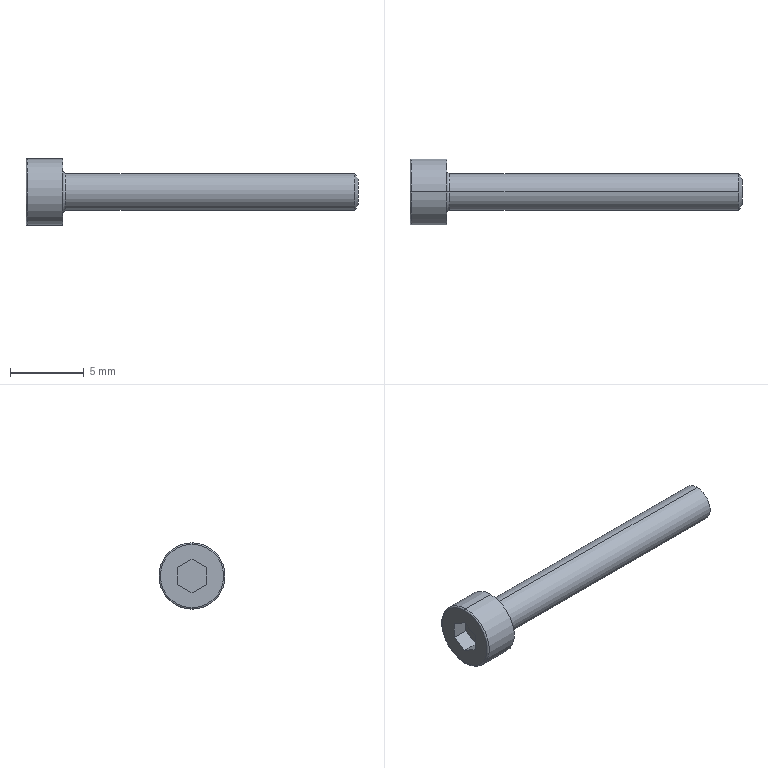Part | SolidWorks | features BlendCut 1, Cut 1, Fillet 1, LPattern 1, RevCut 1, Revolution 1 | 1 solid | 20 faces | box 22.5 x 4.5 x 4.5 mm | volume 133.887 mm3 | plane 10 | torus 4 | cylinder 4 | cone 2 | commonest cylinder face diameters 2.5 x2 4.5 x2
STEP:
#1=CARTESIAN_POINT('',(0.,0.,2.15));
#2=VERTEX_POINT('',#1);
#3=CARTESIAN_POINT('',(0.,0.,-2.15));
#4=VERTEX_POINT('',#3);
#5=CARTESIAN_POINT('',(0.,0.,0.));
#6=DIRECTION('',(-1.,0.,0.));
#7=DIRECTION('',(0.,0.,-1.));
#8=AXIS2_PLACEMENT_3D('',#5,#6,#7);
#9=CIRCLE('',#8,2.15);
#10=EDGE_CURVE('',#2,#4,#9,.T.);
#11=ORIENTED_EDGE('',*,*,#10,.F.);
#12=CARTESIAN_POINT('',(0.1,0.,2.25));
#13=VERTEX_POINT('',#12);
#14=CARTESIAN_POINT('',(0.1,0.,2.15));
#15=DIRECTION('',(0.,1.,0.));
#16=DIRECTION('',(0.,0.,1.));
#17=AXIS2_PLACEMENT_3D('',#14,#15,#16);
#18=CIRCLE('',#17,0.1);
#19=EDGE_CURVE('',#2,#13,#18,.T.);
#20=ORIENTED_EDGE('',*,*,#19,.T.);
#21=CARTESIAN_POINT('',(0.1,0.,-2.25));
#22=VERTEX_POINT('',#21);
#23=CARTESIAN_POINT('',(0.1,0.,0.));
#24=DIRECTION('',(1.,0.,0.));
#25=DIRECTION('',(0.,0.,-1.));
#26=AXIS2_PLACEMENT_3D('',#23,#24,#25);
#27=CIRCLE('',#26,2.25);
#28=EDGE_CURVE('',#22,#13,#27,.T.);
#29=ORIENTED_EDGE('',*,*,#28,.F.);
#30=CARTESIAN_POINT('',(0.1,0.,-2.15));
#31=DIRECTION('',(0.,-1.,0.));
#32=DIRECTION('',(0.,0.,-1.));
#33=AXIS2_PLACEMENT_3D('',#30,#31,#32);
#34=CIRCLE('',#33,0.1);
#35=EDGE_CURVE('',#4,#22,#34,.T.);
#36=ORIENTED_EDGE('',*,*,#35,.F.);
#37=EDGE_LOOP('',(#11,#20,#29,#36));
#38=FACE_OUTER_BOUND('',#37,.T.);
#39=CARTESIAN_POINT('',(0.1,0.,0.));
#40=DIRECTION('',(1.,0.,0.));
#41=DIRECTION('',(0.,0.,-1.));
#42=AXIS2_PLACEMENT_3D('',#39,#40,#41);
#43=TOROIDAL_SURFACE('',#42,2.15,0.1);
#44=ADVANCED_FACE('',(#38),#43,.T.);
#45=CARTESIAN_POINT('',(22.5,0.,0.8603));
#46=VERTEX_POINT('',#45);
#47=CARTESIAN_POINT('',(22.5,0.,-0.8603));
#48=VERTEX_POINT('',#47);
#49=CARTESIAN_POINT('',(22.5,0.,0.));
#50=DIRECTION('',(-1.,0.,0.));
#51=DIRECTION('',(0.,0.,1.));
#52=AXIS2_PLACEMENT_3D('',#49,#50,#51);
#53=CIRCLE('',#52,0.8603);
#54=EDGE_CURVE('',#46,#48,#53,.T.);
#55=ORIENTED_EDGE('',*,*,#54,.T.);
#56=CARTESIAN_POINT('',(22.275,0.,-1.25));
#57=VERTEX_POINT('',#56);
#58=CARTESIAN_POINT('',(22.275,0.,-1.25));
#59=DIRECTION('',(-0.5,0.,-0.866));
#60=VECTOR('',#59,1000.);
#61=LINE('',#58,#60);
#62=EDGE_CURVE('',#48,#57,#61,.T.);
#63=ORIENTED_EDGE('',*,*,#62,.T.);
#64=CARTESIAN_POINT('',(22.275,0.,1.25));
#65=VERTEX_POINT('',#64);
#66=CARTESIAN_POINT('',(22.275,0.,0.));
#67=DIRECTION('',(-1.,0.,0.));
#68=DIRECTION('',(0.,0.,1.));
#69=AXIS2_PLACEMENT_3D('',#66,#67,#68);
#70=CIRCLE('',#69,1.25);
#71=EDGE_CURVE('',#65,#57,#70,.T.);
#72=ORIENTED_EDGE('',*,*,#71,.F.);
#73=CARTESIAN_POINT('',(22.275,0.,1.25));
#74=DIRECTION('',(-0.5,0.,0.866));
#75=VECTOR('',#74,1000.);
#76=LINE('',#73,#75);
#77=EDGE_CURVE('',#46,#65,#76,.T.);
#78=ORIENTED_EDGE('',*,*,#77,.F.);
#79=EDGE_LOOP('',(#55,#63,#72,#78));
#80=FACE_OUTER_BOUND('',#79,.T.);
#81=CARTESIAN_POINT('',(22.275,0.,0.));
#82=DIRECTION('',(-1.,0.,0.));
#83=DIRECTION('',(0.,0.,1.));
#84=AXIS2_PLACEMENT_3D('',#81,#82,#83);
#85=CONICAL_SURFACE('',#84,1.25,1.047);
#86=ADVANCED_FACE('',(#80),#85,.T.);
#87=CARTESIAN_POINT('',(2.5,0.,-1.45));
#88=VERTEX_POINT('',#87);
#89=CARTESIAN_POINT('',(2.5,0.,1.45));
#90=VERTEX_POINT('',#89);
#91=CARTESIAN_POINT('',(2.5,0.,0.));
#92=DIRECTION('',(-1.,0.,0.));
#93=DIRECTION('',(0.,0.,1.));
#94=AXIS2_PLACEMENT_3D('',#91,#92,#93);
#95=CIRCLE('',#94,1.45);
#96=EDGE_CURVE('',#88,#90,#95,.T.);
#97=ORIENTED_EDGE('',*,*,#96,.F.);
#98=CARTESIAN_POINT('',(2.7,0.,-1.25));
#99=VERTEX_POINT('',#98);
#100=CARTESIAN_POINT('',(2.7,0.,-1.45));
#101=DIRECTION('',(0.,1.,0.));
#102=DIRECTION('',(0.,0.,1.));
#103=AXIS2_PLACEMENT_3D('',#100,#101,#102);
#104=CIRCLE('',#103,0.2);
#105=EDGE_CURVE('',#88,#99,#104,.T.);
#106=ORIENTED_EDGE('',*,*,#105,.T.);
#107=CARTESIAN_POINT('',(2.7,0.,1.25));
#108=VERTEX_POINT('',#107);
#109=CARTESIAN_POINT('',(2.7,0.,0.));
#110=DIRECTION('',(-1.,0.,0.));
#111=DIRECTION('',(0.,0.,1.));
#112=AXIS2_PLACEMENT_3D('',#109,#110,#111);
#113=CIRCLE('',#112,1.25);
#114=EDGE_CURVE('',#99,#108,#113,.T.);
#115=ORIENTED_EDGE('',*,*,#114,.T.);
#116=CARTESIAN_POINT('',(2.7,0.,1.45));
#117=DIRECTION('',(0.,-1.,0.));
#118=DIRECTION('',(0.,0.,-1.));
#119=AXIS2_PLACEMENT_3D('',#116,#117,#118);
#120=CIRCLE('',#119,0.2);
#121=EDGE_CURVE('',#90,#108,#120,.T.);
#122=ORIENTED_EDGE('',*,*,#121,.F.);
#123=EDGE_LOOP('',(#97,#106,#115,#122));
#124=FACE_OUTER_BOUND('',#123,.T.);
#125=CARTESIAN_POINT('',(2.7,0.,0.));
#126=DIRECTION('',(-1.,0.,0.));
#127=DIRECTION('',(0.,0.,1.));
#128=AXIS2_PLACEMENT_3D('',#125,#126,#127);
#129=TOROIDAL_SURFACE('',#128,1.45,0.2);
#130=ADVANCED_FACE('',(#124),#129,.F.);
#131=CARTESIAN_POINT('',(2.5,0.,2.25));
#132=VERTEX_POINT('',#131);
#133=CARTESIAN_POINT('',(2.5,0.,-2.25));
#134=VERTEX_POINT('',#133);
#135=CARTESIAN_POINT('',(2.5,0.,0.));
#136=DIRECTION('',(-1.,0.,0.));
#137=DIRECTION('',(0.,0.,1.));
#138=AXIS2_PLACEMENT_3D('',#135,#136,#137);
#139=CIRCLE('',#138,2.25);
#140=EDGE_CURVE('',#132,#134,#139,.T.);
#141=ORIENTED_EDGE('',*,*,#140,.T.);
#142=CARTESIAN_POINT('',(0.,0.,-2.25));
#143=DIRECTION('',(-1.,0.,0.));
#144=VECTOR('',#143,1000.);
#145=LINE('',#142,#144);
#146=EDGE_CURVE('',#134,#22,#145,.T.);
#147=ORIENTED_EDGE('',*,*,#146,.T.);
#148=ORIENTED_EDGE('',*,*,#28,.T.);
#149=CARTESIAN_POINT('',(0.,0.,2.25));
#150=DIRECTION('',(-1.,0.,0.));
#151=VECTOR('',#150,1000.);
#152=LINE('',#149,#151);
#153=EDGE_CURVE('',#132,#13,#152,.T.);
#154=ORIENTED_EDGE('',*,*,#153,.F.);
#155=EDGE_LOOP('',(#141,#147,#148,#154));
#156=FACE_OUTER_BOUND('',#155,.T.);
#157=CARTESIAN_POINT('',(0.,0.,0.));
#158=DIRECTION('',(-1.,0.,0.));
#159=DIRECTION('',(0.,0.,1.));
#160=AXIS2_PLACEMENT_3D('',#157,#158,#159);
#161=CYLINDRICAL_SURFACE('',#160,2.25);
#162=ADVANCED_FACE('',(#156),#161,.T.);
#163=ORIENTED_EDGE('',*,*,#71,.T.);
#164=CARTESIAN_POINT('',(0.,0.,-1.25));
#165=DIRECTION('',(-1.,0.,0.));
#166=VECTOR('',#165,1000.);
#167=LINE('',#164,#166);
#168=EDGE_CURVE('',#57,#99,#167,.T.);
#169=ORIENTED_EDGE('',*,*,#168,.T.);
#170=CARTESIAN_POINT('',(2.7,0.,0.));
#171=DIRECTION('',(-1.,0.,0.));
#172=DIRECTION('',(0.,0.,1.));
#173=AXIS2_PLACEMENT_3D('',#170,#171,#172);
#174=CIRCLE('',#173,1.25);
#175=EDGE_CURVE('',#108,#99,#174,.T.);
#176=ORIENTED_EDGE('',*,*,#175,.F.);
#177=CARTESIAN_POINT('',(0.,0.,1.25));
#178=DIRECTION('',(-1.,0.,0.));
#179=VECTOR('',#178,1000.);
#180=LINE('',#177,#179);
#181=EDGE_CURVE('',#65,#108,#180,.T.);
#182=ORIENTED_EDGE('',*,*,#181,.F.);
#183=EDGE_LOOP('',(#163,#169,#176,#182));
#184=FACE_OUTER_BOUND('',#183,.T.);
#185=CARTESIAN_POINT('',(0.,0.,0.));
#186=DIRECTION('',(-1.,0.,0.));
#187=DIRECTION('',(0.,0.,1.));
#188=AXIS2_PLACEMENT_3D('',#185,#186,#187);
#189=CYLINDRICAL_SURFACE('',#188,1.25);
#190=ADVANCED_FACE('',(#184),#189,.T.);
#191=ORIENTED_EDGE('',*,*,#168,.F.);
#192=CARTESIAN_POINT('',(22.275,0.,0.));
#193=DIRECTION('',(-1.,0.,0.));
#194=DIRECTION('',(0.,0.,1.));
#195=AXIS2_PLACEMENT_3D('',#192,#193,#194);
#196=CIRCLE('',#195,1.25);
#197=EDGE_CURVE('',#57,#65,#196,.T.);
#198=ORIENTED_EDGE('',*,*,#197,.T.);
#199=ORIENTED_EDGE('',*,*,#181,.T.);
#200=ORIENTED_EDGE('',*,*,#114,.F.);
#201=EDGE_LOOP('',(#191,#198,#199,#200));
#202=FACE_OUTER_BOUND('',#201,.T.);
#203=CARTESIAN_POINT('',(0.,0.,0.));
#204=DIRECTION('',(-1.,0.,0.));
#205=DIRECTION('',(0.,0.,1.));
#206=AXIS2_PLACEMENT_3D('',#203,#204,#205);
#207=CYLINDRICAL_SURFACE('',#206,1.25);
#208=ADVANCED_FACE('',(#202),#207,.T.);
#209=CARTESIAN_POINT('',(0.,0.,0.));
#210=DIRECTION('',(-1.,0.,0.));
#211=DIRECTION('',(0.,0.,-1.));
#212=AXIS2_PLACEMENT_3D('',#209,#210,#211);
#213=CIRCLE('',#212,2.15);
#214=EDGE_CURVE('',#4,#2,#213,.T.);
#215=ORIENTED_EDGE('',*,*,#214,.T.);
#216=ORIENTED_EDGE('',*,*,#10,.T.);
#217=EDGE_LOOP('',(#215,#216));
#218=FACE_OUTER_BOUND('',#217,.T.);
#219=CARTESIAN_POINT('',(0.,0.,1.15));
#220=VERTEX_POINT('',#219);
#221=CARTESIAN_POINT('',(0.,0.9959,0.575));
#222=VERTEX_POINT('',#221);
#223=CARTESIAN_POINT('',(0.,0.,1.15));
#224=DIRECTION('',(0.,0.866,-0.5));
#225=VECTOR('',#224,1000.);
#226=LINE('',#223,#225);
#227=EDGE_CURVE('',#220,#222,#226,.T.);
#228=ORIENTED_EDGE('',*,*,#227,.F.);
#229=CARTESIAN_POINT('',(0.,-0.9959,0.575));
#230=VERTEX_POINT('',#229);
#231=CARTESIAN_POINT('',(0.,-0.9959,0.575));
#232=DIRECTION('',(0.,0.866,0.5));
#233=VECTOR('',#232,1000.);
#234=LINE('',#231,#233);
#235=EDGE_CURVE('',#230,#220,#234,.T.);
#236=ORIENTED_EDGE('',*,*,#235,.F.);
#237=CARTESIAN_POINT('',(0.,-0.9959,-0.575));
#238=VERTEX_POINT('',#237);
#239=CARTESIAN_POINT('',(0.,-0.9959,-0.575));
#240=DIRECTION('',(0.,0.,1.));
#241=VECTOR('',#240,1000.);
#242=LINE('',#239,#241);
#243=EDGE_CURVE('',#238,#230,#242,.T.);
#244=ORIENTED_EDGE('',*,*,#243,.F.);
#245=CARTESIAN_POINT('',(0.,0.,-1.15));
#246=VERTEX_POINT('',#245);
#247=CARTESIAN_POINT('',(0.,0.,-1.15));
#248=DIRECTION('',(0.,-0.866,0.5));
#249=VECTOR('',#248,1000.);
#250=LINE('',#247,#249);
#251=EDGE_CURVE('',#246,#238,#250,.T.);
#252=ORIENTED_EDGE('',*,*,#251,.F.);
#253=CARTESIAN_POINT('',(0.,0.9959,-0.575));
#254=VERTEX_POINT('',#253);
#255=CARTESIAN_POINT('',(0.,0.9959,-0.575));
#256=DIRECTION('',(0.,-0.866,-0.5));
#257=VECTOR('',#256,1000.);
#258=LINE('',#255,#257);
#259=EDGE_CURVE('',#254,#246,#258,.T.);
#260=ORIENTED_EDGE('',*,*,#259,.F.);
#261=CARTESIAN_POINT('',(0.,0.9959,0.575));
#262=DIRECTION('',(0.,0.,-1.));
#263=VECTOR('',#262,1000.);
#264=LINE('',#261,#263);
#265=EDGE_CURVE('',#222,#254,#264,.T.);
#266=ORIENTED_EDGE('',*,*,#265,.F.);
#267=EDGE_LOOP('',(#228,#236,#244,#252,#260,#266));
#268=FACE_BOUND('',#267,.T.);
#269=CARTESIAN_POINT('',(0.,0.,0.));
#270=DIRECTION('',(1.,0.,0.));
#271=DIRECTION('',(0.,0.,-1.));
#272=AXIS2_PLACEMENT_3D('',#269,#270,#271);
#273=PLANE('',#272);
#274=ADVANCED_FACE('',(#218,#268),#273,.F.);
#275=ORIENTED_EDGE('',*,*,#146,.F.);
#276=CARTESIAN_POINT('',(2.5,0.,0.));
#277=DIRECTION('',(-1.,0.,0.));
#278=DIRECTION('',(0.,0.,1.));
#279=AXIS2_PLACEMENT_3D('',#276,#277,#278);
#280=CIRCLE('',#279,2.25);
#281=EDGE_CURVE('',#134,#132,#280,.T.);
#282=ORIENTED_EDGE('',*,*,#281,.T.);
#283=ORIENTED_EDGE('',*,*,#153,.T.);
#284=CARTESIAN_POINT('',(0.1,0.,0.));
#285=DIRECTION('',(1.,0.,0.));
#286=DIRECTION('',(0.,0.,-1.));
#287=AXIS2_PLACEMENT_3D('',#284,#285,#286);
#288=CIRCLE('',#287,2.25);
#289=EDGE_CURVE('',#13,#22,#288,.T.);
#290=ORIENTED_EDGE('',*,*,#289,.T.);
#291=EDGE_LOOP('',(#275,#282,#283,#290));
#292=FACE_OUTER_BOUND('',#291,.T.);
#293=CARTESIAN_POINT('',(0.,0.,0.));
#294=DIRECTION('',(-1.,0.,0.));
#295=DIRECTION('',(0.,0.,1.));
#296=AXIS2_PLACEMENT_3D('',#293,#294,#295);
#297=CYLINDRICAL_SURFACE('',#296,2.25);
#298=ADVANCED_FACE('',(#292),#297,.T.);
#299=ORIENTED_EDGE('',*,*,#140,.F.);
#300=ORIENTED_EDGE('',*,*,#281,.F.);
#301=EDGE_LOOP('',(#299,#300));
#302=FACE_OUTER_BOUND('',#301,.T.);
#303=CARTESIAN_POINT('',(2.5,0.,0.));
#304=DIRECTION('',(-1.,0.,0.));
#305=DIRECTION('',(0.,0.,1.));
#306=AXIS2_PLACEMENT_3D('',#303,#304,#305);
#307=CIRCLE('',#306,1.45);
#308=EDGE_CURVE('',#90,#88,#307,.T.);
#309=ORIENTED_EDGE('',*,*,#308,.T.);
#310=ORIENTED_EDGE('',*,*,#96,.T.);
#311=EDGE_LOOP('',(#309,#310));
#312=FACE_BOUND('',#311,.T.);
#313=CARTESIAN_POINT('',(2.5,2.25,0.));
#314=DIRECTION('',(-1.,0.,0.));
#315=DIRECTION('',(0.,0.,1.));
#316=AXIS2_PLACEMENT_3D('',#313,#314,#315);
#317=PLANE('',#316);
#318=ADVANCED_FACE('',(#302,#312),#317,.F.);
#319=ORIENTED_EDGE('',*,*,#105,.F.);
#320=ORIENTED_EDGE('',*,*,#308,.F.);
#321=ORIENTED_EDGE('',*,*,#121,.T.);
#322=ORIENTED_EDGE('',*,*,#175,.T.);
#323=EDGE_LOOP('',(#319,#320,#321,#322));
#324=FACE_OUTER_BOUND('',#323,.T.);
#325=CARTESIAN_POINT('',(2.7,0.,0.));
#326=DIRECTION('',(-1.,0.,0.));
#327=DIRECTION('',(0.,0.,1.));
#328=AXIS2_PLACEMENT_3D('',#325,#326,#327);
#329=TOROIDAL_SURFACE('',#328,1.45,0.2);
#330=ADVANCED_FACE('',(#324),#329,.F.);
#331=ORIENTED_EDGE('',*,*,#235,.T.);
#332=CARTESIAN_POINT('',(1.1,0.,1.15));
#333=VERTEX_POINT('',#332);
#334=CARTESIAN_POINT('',(1.1,0.,1.15));
#335=DIRECTION('',(-1.,0.,0.));
#336=VECTOR('',#335,1000.);
#337=LINE('',#334,#336);
#338=EDGE_CURVE('',#333,#220,#337,.T.);
#339=ORIENTED_EDGE('',*,*,#338,.F.);
#340=CARTESIAN_POINT('',(1.1,-0.9959,0.575));
#341=VERTEX_POINT('',#340);
#342=CARTESIAN_POINT('',(1.1,-0.9959,0.575));
#343=DIRECTION('',(0.,0.866,0.5));
#344=VECTOR('',#343,1000.);
#345=LINE('',#342,#344);
#346=EDGE_CURVE('',#341,#333,#345,.T.);
#347=ORIENTED_EDGE('',*,*,#346,.F.);
#348=CARTESIAN_POINT('',(1.1,-0.9959,0.575));
#349=DIRECTION('',(-1.,0.,0.));
#350=VECTOR('',#349,1000.);
#351=LINE('',#348,#350);
#352=EDGE_CURVE('',#341,#230,#351,.T.);
#353=ORIENTED_EDGE('',*,*,#352,.T.);
#354=EDGE_LOOP('',(#331,#339,#347,#353));
#355=FACE_OUTER_BOUND('',#354,.T.);
#356=CARTESIAN_POINT('',(1.1,-0.9959,0.575));
#357=DIRECTION('',(0.,-0.5,0.866));
#358=DIRECTION('',(0.,-0.866,-0.5));
#359=AXIS2_PLACEMENT_3D('',#356,#357,#358);
#360=PLANE('',#359);
#361=ADVANCED_FACE('',(#355),#360,.F.);
#362=ORIENTED_EDGE('',*,*,#243,.T.);
#363=ORIENTED_EDGE('',*,*,#352,.F.);
#364=CARTESIAN_POINT('',(1.1,-0.9959,-0.575));
#365=VERTEX_POINT('',#364);
#366=CARTESIAN_POINT('',(1.1,-0.9959,-0.575));
#367=DIRECTION('',(0.,0.,1.));
#368=VECTOR('',#367,1000.);
#369=LINE('',#366,#368);
#370=EDGE_CURVE('',#365,#341,#369,.T.);
#371=ORIENTED_EDGE('',*,*,#370,.F.);
#372=CARTESIAN_POINT('',(1.1,-0.9959,-0.575));
#373=DIRECTION('',(-1.,0.,0.));
#374=VECTOR('',#373,1000.);
#375=LINE('',#372,#374);
#376=EDGE_CURVE('',#365,#238,#375,.T.);
#377=ORIENTED_EDGE('',*,*,#376,.T.);
#378=EDGE_LOOP('',(#362,#363,#371,#377));
#379=FACE_OUTER_BOUND('',#378,.T.);
#380=CARTESIAN_POINT('',(1.1,-0.9959,-0.575));
#381=DIRECTION('',(0.,-1.,0.));
#382=DIRECTION('',(0.,0.,-1.));
#383=AXIS2_PLACEMENT_3D('',#380,#381,#382);
#384=PLANE('',#383);
#385=ADVANCED_FACE('',(#379),#384,.F.);
#386=ORIENTED_EDGE('',*,*,#251,.T.);
#387=ORIENTED_EDGE('',*,*,#376,.F.);
#388=CARTESIAN_POINT('',(1.1,0.,-1.15));
#389=VERTEX_POINT('',#388);
#390=CARTESIAN_POINT('',(1.1,0.,-1.15));
#391=DIRECTION('',(0.,-0.866,0.5));
#392=VECTOR('',#391,1000.);
#393=LINE('',#390,#392);
#394=EDGE_CURVE('',#389,#365,#393,.T.);
#395=ORIENTED_EDGE('',*,*,#394,.F.);
#396=CARTESIAN_POINT('',(1.1,0.,-1.15));
#397=DIRECTION('',(-1.,0.,0.));
#398=VECTOR('',#397,1000.);
#399=LINE('',#396,#398);
#400=EDGE_CURVE('',#389,#246,#399,.T.);
#401=ORIENTED_EDGE('',*,*,#400,.T.);
#402=EDGE_LOOP('',(#386,#387,#395,#401));
#403=FACE_OUTER_BOUND('',#402,.T.);
#404=CARTESIAN_POINT('',(1.1,0.,-1.15));
#405=DIRECTION('',(0.,-0.5,-0.866));
#406=DIRECTION('',(0.,0.866,-0.5));
#407=AXIS2_PLACEMENT_3D('',#404,#405,#406);
#408=PLANE('',#407);
#409=ADVANCED_FACE('',(#403),#408,.F.);
#410=ORIENTED_EDGE('',*,*,#259,.T.);
#411=ORIENTED_EDGE('',*,*,#400,.F.);
#412=CARTESIAN_POINT('',(1.1,0.9959,-0.575));
#413=VERTEX_POINT('',#412);
#414=CARTESIAN_POINT('',(1.1,0.9959,-0.575));
#415=DIRECTION('',(0.,-0.866,-0.5));
#416=VECTOR('',#415,1000.);
#417=LINE('',#414,#416);
#418=EDGE_CURVE('',#413,#389,#417,.T.);
#419=ORIENTED_EDGE('',*,*,#418,.F.);
#420=CARTESIAN_POINT('',(1.1,0.9959,-0.575));
#421=DIRECTION('',(-1.,0.,0.));
#422=VECTOR('',#421,1000.);
#423=LINE('',#420,#422);
#424=EDGE_CURVE('',#413,#254,#423,.T.);
#425=ORIENTED_EDGE('',*,*,#424,.T.);
#426=EDGE_LOOP('',(#410,#411,#419,#425));
#427=FACE_OUTER_BOUND('',#426,.T.);
#428=CARTESIAN_POINT('',(1.1,0.9959,-0.575));
#429=DIRECTION('',(0.,0.5,-0.866));
#430=DIRECTION('',(0.,0.866,0.5));
#431=AXIS2_PLACEMENT_3D('',#428,#429,#430);
#432=PLANE('',#431);
#433=ADVANCED_FACE('',(#427),#432,.F.);
#434=ORIENTED_EDGE('',*,*,#265,.T.);
#435=ORIENTED_EDGE('',*,*,#424,.F.);
#436=CARTESIAN_POINT('',(1.1,0.9959,0.575));
#437=VERTEX_POINT('',#436);
#438=CARTESIAN_POINT('',(1.1,0.9959,0.575));
#439=DIRECTION('',(0.,0.,-1.));
#440=VECTOR('',#439,1000.);
#441=LINE('',#438,#440);
#442=EDGE_CURVE('',#437,#413,#441,.T.);
#443=ORIENTED_EDGE('',*,*,#442,.F.);
#444=CARTESIAN_POINT('',(1.1,0.9959,0.575));
#445=DIRECTION('',(-1.,0.,0.));
#446=VECTOR('',#445,1000.);
#447=LINE('',#444,#446);
#448=EDGE_CURVE('',#437,#222,#447,.T.);
#449=ORIENTED_EDGE('',*,*,#448,.T.);
#450=EDGE_LOOP('',(#434,#435,#443,#449));
#451=FACE_OUTER_BOUND('',#450,.T.);
#452=CARTESIAN_POINT('',(1.1,0.9959,0.575));
#453=DIRECTION('',(0.,1.,0.));
#454=DIRECTION('',(0.,0.,1.));
#455=AXIS2_PLACEMENT_3D('',#452,#453,#454);
#456=PLANE('',#455);
#457=ADVANCED_FACE('',(#451),#456,.F.);
#458=ORIENTED_EDGE('',*,*,#227,.T.);
#459=ORIENTED_EDGE('',*,*,#448,.F.);
#460=CARTESIAN_POINT('',(1.1,0.,1.15));
#461=DIRECTION('',(0.,0.866,-0.5));
#462=VECTOR('',#461,1000.);
#463=LINE('',#460,#462);
#464=EDGE_CURVE('',#333,#437,#463,.T.);
#465=ORIENTED_EDGE('',*,*,#464,.F.);
#466=ORIENTED_EDGE('',*,*,#338,.T.);
#467=EDGE_LOOP('',(#458,#459,#465,#466));
#468=FACE_OUTER_BOUND('',#467,.T.);
#469=CARTESIAN_POINT('',(1.1,0.,1.15));
#470=DIRECTION('',(0.,0.5,0.866));
#471=DIRECTION('',(0.,-0.866,0.5));
#472=AXIS2_PLACEMENT_3D('',#469,#470,#471);
#473=PLANE('',#472);
#474=ADVANCED_FACE('',(#468),#473,.F.);
#475=ORIENTED_EDGE('',*,*,#346,.T.);
#476=ORIENTED_EDGE('',*,*,#464,.T.);
#477=ORIENTED_EDGE('',*,*,#442,.T.);
#478=ORIENTED_EDGE('',*,*,#418,.T.);
#479=ORIENTED_EDGE('',*,*,#394,.T.);
#480=ORIENTED_EDGE('',*,*,#370,.T.);
#481=EDGE_LOOP('',(#475,#476,#477,#478,#479,#480));
#482=FACE_OUTER_BOUND('',#481,.T.);
#483=CARTESIAN_POINT('',(1.1,-0.9959,0.575));
#484=DIRECTION('',(1.,0.,0.));
#485=DIRECTION('',(0.,0.,-1.));
#486=AXIS2_PLACEMENT_3D('',#483,#484,#485);
#487=PLANE('',#486);
#488=ADVANCED_FACE('',(#482),#487,.F.);
#489=ORIENTED_EDGE('',*,*,#62,.F.);
#490=CARTESIAN_POINT('',(22.5,0.,0.));
#491=DIRECTION('',(-1.,0.,0.));
#492=DIRECTION('',(0.,0.,1.));
#493=AXIS2_PLACEMENT_3D('',#490,#491,#492);
#494=CIRCLE('',#493,0.8603);
#495=EDGE_CURVE('',#48,#46,#494,.T.);
#496=ORIENTED_EDGE('',*,*,#495,.T.);
#497=ORIENTED_EDGE('',*,*,#77,.T.);
#498=ORIENTED_EDGE('',*,*,#197,.F.);
#499=EDGE_LOOP('',(#489,#496,#497,#498));
#500=FACE_OUTER_BOUND('',#499,.T.);
#501=CARTESIAN_POINT('',(22.275,0.,0.));
#502=DIRECTION('',(-1.,0.,0.));
#503=DIRECTION('',(0.,0.,1.));
#504=AXIS2_PLACEMENT_3D('',#501,#502,#503);
#505=CONICAL_SURFACE('',#504,1.25,1.047);
#506=ADVANCED_FACE('',(#500),#505,.T.);
#507=ORIENTED_EDGE('',*,*,#54,.F.);
#508=ORIENTED_EDGE('',*,*,#495,.F.);
#509=EDGE_LOOP('',(#507,#508));
#510=FACE_OUTER_BOUND('',#509,.T.);
#511=CARTESIAN_POINT('',(22.5,1.25,0.));
#512=DIRECTION('',(-1.,0.,0.));
#513=DIRECTION('',(0.,0.,1.));
#514=AXIS2_PLACEMENT_3D('',#511,#512,#513);
#515=PLANE('',#514);
#516=ADVANCED_FACE('',(#510),#515,.F.);
#517=ORIENTED_EDGE('',*,*,#19,.F.);
#518=ORIENTED_EDGE('',*,*,#214,.F.);
#519=ORIENTED_EDGE('',*,*,#35,.T.);
#520=ORIENTED_EDGE('',*,*,#289,.F.);
#521=EDGE_LOOP('',(#517,#518,#519,#520));
#522=FACE_OUTER_BOUND('',#521,.T.);
#523=CARTESIAN_POINT('',(0.1,0.,0.));
#524=DIRECTION('',(1.,0.,0.));
#525=DIRECTION('',(0.,0.,-1.));
#526=AXIS2_PLACEMENT_3D('',#523,#524,#525);
#527=TOROIDAL_SURFACE('',#526,2.15,0.1);
#528=ADVANCED_FACE('',(#522),#527,.T.);
#529=CLOSED_SHELL('',(#44,#86,#130,#162,#190,#208,#274,#298,#318,#330,#361,#385,#409,#433,#457,#474,#488,#506,#516,#528));
#530=MANIFOLD_SOLID_BREP('',#529);
#531=CARTESIAN_POINT('',(0.,0.,0.));
#532=DIRECTION('',(0.,0.,1.));
#533=DIRECTION('',(1.,0.,0.));
#534=AXIS2_PLACEMENT_3D('',#531,#532,#533);
#535=(LENGTH_UNIT()NAMED_UNIT(*)SI_UNIT(.MILLI.,.METRE.));
#536=UNCERTAINTY_MEASURE_WITH_UNIT(LENGTH_MEASURE(0.00001),#535,'','');
#537=(NAMED_UNIT(*)PLANE_ANGLE_UNIT()SI_UNIT($,.RADIAN.));
#538=(NAMED_UNIT(*)SI_UNIT($,.STERADIAN.)SOLID_ANGLE_UNIT());
#539=(GEOMETRIC_REPRESENTATION_CONTEXT(3)GLOBAL_UNCERTAINTY_ASSIGNED_CONTEXT((#536))GLOBAL_UNIT_ASSIGNED_CONTEXT((#535,#537,#538))REPRESENTATION_CONTEXT('',''));
#540=ADVANCED_BREP_SHAPE_REPRESENTATION('',(#530,#534),#539);